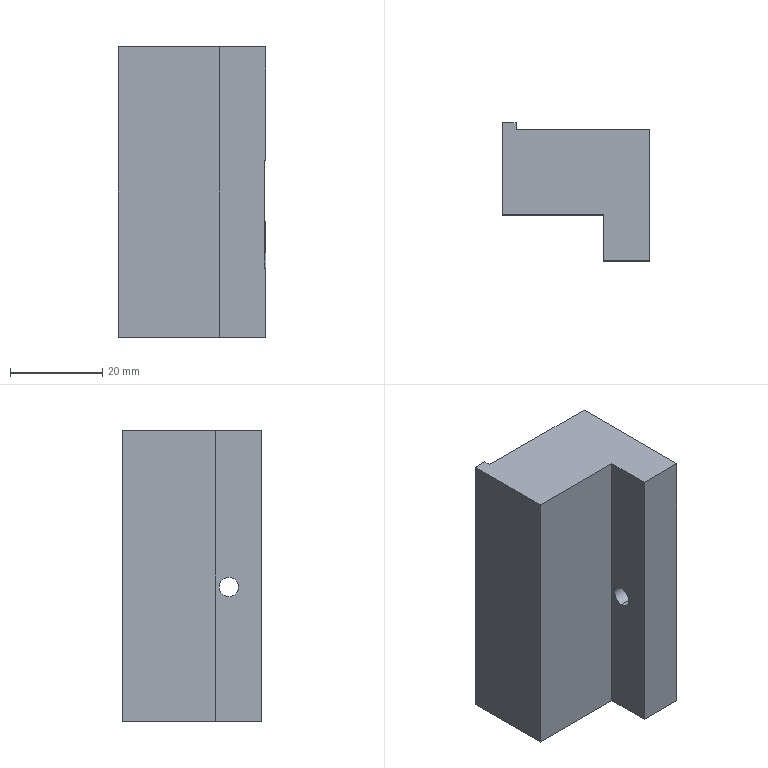Part | SolidWorks | features ICE 2, 3DProfileFeature 1, Extrusion 1, HoleWzd 1 | 1 solid | 16 faces | box 32 x 30 x 63 mm | volume 43546 mm3 | plane 14 | cylinder 2 | commonest cylinder face diameters 4.2 x2
STEP:
#1=CARTESIAN_POINT('',(22.,-23.,-0.2864));
#2=VERTEX_POINT('',#1);
#3=CARTESIAN_POINT('',(22.,-23.,-4.486));
#4=VERTEX_POINT('',#3);
#5=CARTESIAN_POINT('',(22.,-23.,-2.386));
#6=DIRECTION('',(1.,0.,0.));
#7=DIRECTION('',(0.,0.,-1.));
#8=AXIS2_PLACEMENT_3D('',#5,#6,#7);
#9=CIRCLE('',#8,2.1);
#10=EDGE_CURVE('',#2,#4,#9,.T.);
#11=ORIENTED_EDGE('',*,*,#10,.F.);
#12=CARTESIAN_POINT('',(31.7,-23.,-0.2864));
#13=VERTEX_POINT('',#12);
#14=CARTESIAN_POINT('',(31.7,-23.,-0.2864));
#15=DIRECTION('',(1.,0.,0.));
#16=VECTOR('',#15,1000.);
#17=LINE('',#14,#16);
#18=EDGE_CURVE('',#2,#13,#17,.T.);
#19=ORIENTED_EDGE('',*,*,#18,.T.);
#20=CARTESIAN_POINT('',(31.7,-23.,-4.486));
#21=VERTEX_POINT('',#20);
#22=CARTESIAN_POINT('',(31.7,-23.,-2.386));
#23=DIRECTION('',(1.,0.,0.));
#24=DIRECTION('',(0.,0.,-1.));
#25=AXIS2_PLACEMENT_3D('',#22,#23,#24);
#26=CIRCLE('',#25,2.1);
#27=EDGE_CURVE('',#13,#21,#26,.T.);
#28=ORIENTED_EDGE('',*,*,#27,.T.);
#29=CARTESIAN_POINT('',(31.7,-23.,-4.486));
#30=DIRECTION('',(1.,0.,0.));
#31=VECTOR('',#30,1000.);
#32=LINE('',#29,#31);
#33=EDGE_CURVE('',#4,#21,#32,.T.);
#34=ORIENTED_EDGE('',*,*,#33,.F.);
#35=EDGE_LOOP('',(#11,#19,#28,#34));
#36=FACE_OUTER_BOUND('',#35,.T.);
#37=CARTESIAN_POINT('',(31.7,-23.,-2.386));
#38=DIRECTION('',(1.,0.,0.));
#39=DIRECTION('',(0.,0.,-1.));
#40=AXIS2_PLACEMENT_3D('',#37,#38,#39);
#41=CYLINDRICAL_SURFACE('',#40,2.1);
#42=ADVANCED_FACE('',(#36),#41,.F.);
#43=CARTESIAN_POINT('',(32.,-1.5,-6.5));
#44=VERTEX_POINT('',#43);
#45=CARTESIAN_POINT('',(32.,-1.5,-31.5));
#46=VERTEX_POINT('',#45);
#47=CARTESIAN_POINT('',(32.,-1.5,-31.5));
#48=DIRECTION('',(0.,0.,-1.));
#49=VECTOR('',#48,1000.);
#50=LINE('',#47,#49);
#51=EDGE_CURVE('',#44,#46,#50,.T.);
#52=ORIENTED_EDGE('',*,*,#51,.F.);
#53=CARTESIAN_POINT('',(32.,-30.,-16.5));
#54=VERTEX_POINT('',#53);
#55=CARTESIAN_POINT('',(32.,-1.5,-6.5));
#56=DIRECTION('',(0.,0.9436,0.3311));
#57=VECTOR('',#56,1000.);
#58=LINE('',#55,#57);
#59=EDGE_CURVE('',#54,#44,#58,.T.);
#60=ORIENTED_EDGE('',*,*,#59,.F.);
#61=CARTESIAN_POINT('',(32.,-30.,-31.5));
#62=VERTEX_POINT('',#61);
#63=CARTESIAN_POINT('',(32.,-30.,31.5));
#64=DIRECTION('',(0.,0.,-1.));
#65=VECTOR('',#64,1000.);
#66=LINE('',#63,#65);
#67=EDGE_CURVE('',#54,#62,#66,.T.);
#68=ORIENTED_EDGE('',*,*,#67,.T.);
#69=CARTESIAN_POINT('',(32.,0.,-31.5));
#70=DIRECTION('',(0.,1.,0.));
#71=VECTOR('',#70,1000.);
#72=LINE('',#69,#71);
#73=EDGE_CURVE('',#62,#46,#72,.T.);
#74=ORIENTED_EDGE('',*,*,#73,.T.);
#75=EDGE_LOOP('',(#52,#60,#68,#74));
#76=FACE_OUTER_BOUND('',#75,.T.);
#77=CARTESIAN_POINT('',(32.,0.,31.5));
#78=DIRECTION('',(-1.,0.,0.));
#79=DIRECTION('',(0.,0.,1.));
#80=AXIS2_PLACEMENT_3D('',#77,#78,#79);
#81=PLANE('',#80);
#82=ADVANCED_FACE('',(#76),#81,.F.);
#83=CARTESIAN_POINT('',(0.,0.,-31.5));
#84=VERTEX_POINT('',#83);
#85=CARTESIAN_POINT('',(0.,-20.,-31.5));
#86=VERTEX_POINT('',#85);
#87=CARTESIAN_POINT('',(0.,-20.,-31.5));
#88=DIRECTION('',(0.,-1.,0.));
#89=VECTOR('',#88,1000.);
#90=LINE('',#87,#89);
#91=EDGE_CURVE('',#84,#86,#90,.T.);
#92=ORIENTED_EDGE('',*,*,#91,.T.);
#93=CARTESIAN_POINT('',(0.,-20.,31.5));
#94=VERTEX_POINT('',#93);
#95=CARTESIAN_POINT('',(0.,-20.,31.5));
#96=DIRECTION('',(0.,0.,-1.));
#97=VECTOR('',#96,1000.);
#98=LINE('',#95,#97);
#99=EDGE_CURVE('',#94,#86,#98,.T.);
#100=ORIENTED_EDGE('',*,*,#99,.F.);
#101=CARTESIAN_POINT('',(0.,0.,31.5));
#102=VERTEX_POINT('',#101);
#103=CARTESIAN_POINT('',(0.,-20.,31.5));
#104=DIRECTION('',(0.,-1.,0.));
#105=VECTOR('',#104,1000.);
#106=LINE('',#103,#105);
#107=EDGE_CURVE('',#102,#94,#106,.T.);
#108=ORIENTED_EDGE('',*,*,#107,.F.);
#109=CARTESIAN_POINT('',(0.,0.,31.5));
#110=DIRECTION('',(0.,0.,-1.));
#111=VECTOR('',#110,1000.);
#112=LINE('',#109,#111);
#113=EDGE_CURVE('',#102,#84,#112,.T.);
#114=ORIENTED_EDGE('',*,*,#113,.T.);
#115=EDGE_LOOP('',(#92,#100,#108,#114));
#116=FACE_OUTER_BOUND('',#115,.T.);
#117=CARTESIAN_POINT('',(0.,-20.,31.5));
#118=DIRECTION('',(1.,0.,0.));
#119=DIRECTION('',(0.,0.,-1.));
#120=AXIS2_PLACEMENT_3D('',#117,#118,#119);
#121=PLANE('',#120);
#122=ADVANCED_FACE('',(#116),#121,.F.);
#123=CARTESIAN_POINT('',(22.,-20.,-31.5));
#124=VERTEX_POINT('',#123);
#125=CARTESIAN_POINT('',(22.,-20.,-31.5));
#126=DIRECTION('',(1.,0.,0.));
#127=VECTOR('',#126,1000.);
#128=LINE('',#125,#127);
#129=EDGE_CURVE('',#86,#124,#128,.T.);
#130=ORIENTED_EDGE('',*,*,#129,.T.);
#131=CARTESIAN_POINT('',(22.,-20.,31.5));
#132=VERTEX_POINT('',#131);
#133=CARTESIAN_POINT('',(22.,-20.,31.5));
#134=DIRECTION('',(0.,0.,-1.));
#135=VECTOR('',#134,1000.);
#136=LINE('',#133,#135);
#137=EDGE_CURVE('',#132,#124,#136,.T.);
#138=ORIENTED_EDGE('',*,*,#137,.F.);
#139=CARTESIAN_POINT('',(22.,-20.,31.5));
#140=DIRECTION('',(1.,0.,0.));
#141=VECTOR('',#140,1000.);
#142=LINE('',#139,#141);
#143=EDGE_CURVE('',#94,#132,#142,.T.);
#144=ORIENTED_EDGE('',*,*,#143,.F.);
#145=ORIENTED_EDGE('',*,*,#99,.T.);
#146=EDGE_LOOP('',(#130,#138,#144,#145));
#147=FACE_OUTER_BOUND('',#146,.T.);
#148=CARTESIAN_POINT('',(22.,-20.,31.5));
#149=DIRECTION('',(0.,1.,0.));
#150=DIRECTION('',(-1.,0.,0.));
#151=AXIS2_PLACEMENT_3D('',#148,#149,#150);
#152=PLANE('',#151);
#153=ADVANCED_FACE('',(#147),#152,.F.);
#154=CARTESIAN_POINT('',(22.,-23.,-2.386));
#155=DIRECTION('',(1.,0.,0.));
#156=DIRECTION('',(0.,0.,-1.));
#157=AXIS2_PLACEMENT_3D('',#154,#155,#156);
#158=CIRCLE('',#157,2.1);
#159=EDGE_CURVE('',#4,#2,#158,.T.);
#160=ORIENTED_EDGE('',*,*,#159,.T.);
#161=ORIENTED_EDGE('',*,*,#10,.T.);
#162=EDGE_LOOP('',(#160,#161));
#163=FACE_BOUND('',#162,.T.);
#164=CARTESIAN_POINT('',(22.,-30.,-31.5));
#165=VERTEX_POINT('',#164);
#166=CARTESIAN_POINT('',(22.,-30.,-31.5));
#167=DIRECTION('',(0.,-1.,0.));
#168=VECTOR('',#167,1000.);
#169=LINE('',#166,#168);
#170=EDGE_CURVE('',#124,#165,#169,.T.);
#171=ORIENTED_EDGE('',*,*,#170,.T.);
#172=CARTESIAN_POINT('',(22.,-30.,31.5));
#173=VERTEX_POINT('',#172);
#174=CARTESIAN_POINT('',(22.,-30.,31.5));
#175=DIRECTION('',(0.,0.,-1.));
#176=VECTOR('',#175,1000.);
#177=LINE('',#174,#176);
#178=EDGE_CURVE('',#173,#165,#177,.T.);
#179=ORIENTED_EDGE('',*,*,#178,.F.);
#180=CARTESIAN_POINT('',(22.,-30.,31.5));
#181=DIRECTION('',(0.,-1.,0.));
#182=VECTOR('',#181,1000.);
#183=LINE('',#180,#182);
#184=EDGE_CURVE('',#132,#173,#183,.T.);
#185=ORIENTED_EDGE('',*,*,#184,.F.);
#186=ORIENTED_EDGE('',*,*,#137,.T.);
#187=EDGE_LOOP('',(#171,#179,#185,#186));
#188=FACE_OUTER_BOUND('',#187,.T.);
#189=CARTESIAN_POINT('',(22.,-30.,31.5));
#190=DIRECTION('',(1.,0.,0.));
#191=DIRECTION('',(0.,0.,-1.));
#192=AXIS2_PLACEMENT_3D('',#189,#190,#191);
#193=PLANE('',#192);
#194=ADVANCED_FACE('',(#163,#188),#193,.F.);
#195=ORIENTED_EDGE('',*,*,#67,.F.);
#196=CARTESIAN_POINT('',(31.7,-30.,-16.5));
#197=VERTEX_POINT('',#196);
#198=CARTESIAN_POINT('',(31.7,-30.,-16.5));
#199=DIRECTION('',(1.,0.,0.));
#200=VECTOR('',#199,1000.);
#201=LINE('',#198,#200);
#202=EDGE_CURVE('',#197,#54,#201,.T.);
#203=ORIENTED_EDGE('',*,*,#202,.F.);
#204=CARTESIAN_POINT('',(31.7,-30.,6.815));
#205=VERTEX_POINT('',#204);
#206=CARTESIAN_POINT('',(31.7,-30.,-16.5));
#207=DIRECTION('',(0.,0.,-1.));
#208=VECTOR('',#207,1000.);
#209=LINE('',#206,#208);
#210=EDGE_CURVE('',#205,#197,#209,.T.);
#211=ORIENTED_EDGE('',*,*,#210,.F.);
#212=CARTESIAN_POINT('',(32.,-30.,6.815));
#213=VERTEX_POINT('',#212);
#214=CARTESIAN_POINT('',(31.7,-30.,6.815));
#215=DIRECTION('',(1.,0.,0.));
#216=VECTOR('',#215,1000.);
#217=LINE('',#214,#216);
#218=EDGE_CURVE('',#205,#213,#217,.T.);
#219=ORIENTED_EDGE('',*,*,#218,.T.);
#220=CARTESIAN_POINT('',(32.,-30.,31.5));
#221=VERTEX_POINT('',#220);
#222=CARTESIAN_POINT('',(32.,-30.,31.5));
#223=DIRECTION('',(0.,0.,-1.));
#224=VECTOR('',#223,1000.);
#225=LINE('',#222,#224);
#226=EDGE_CURVE('',#221,#213,#225,.T.);
#227=ORIENTED_EDGE('',*,*,#226,.F.);
#228=CARTESIAN_POINT('',(32.,-30.,31.5));
#229=DIRECTION('',(1.,0.,0.));
#230=VECTOR('',#229,1000.);
#231=LINE('',#228,#230);
#232=EDGE_CURVE('',#173,#221,#231,.T.);
#233=ORIENTED_EDGE('',*,*,#232,.F.);
#234=ORIENTED_EDGE('',*,*,#178,.T.);
#235=CARTESIAN_POINT('',(32.,-30.,-31.5));
#236=DIRECTION('',(1.,0.,0.));
#237=VECTOR('',#236,1000.);
#238=LINE('',#235,#237);
#239=EDGE_CURVE('',#165,#62,#238,.T.);
#240=ORIENTED_EDGE('',*,*,#239,.T.);
#241=EDGE_LOOP('',(#195,#203,#211,#219,#227,#233,#234,#240));
#242=FACE_OUTER_BOUND('',#241,.T.);
#243=CARTESIAN_POINT('',(32.,-30.,31.5));
#244=DIRECTION('',(0.,1.,0.));
#245=DIRECTION('',(0.,0.,1.));
#246=AXIS2_PLACEMENT_3D('',#243,#244,#245);
#247=PLANE('',#246);
#248=ADVANCED_FACE('',(#242),#247,.F.);
#249=ORIENTED_EDGE('',*,*,#226,.T.);
#250=CARTESIAN_POINT('',(32.,-1.5,16.815));
#251=VERTEX_POINT('',#250);
#252=CARTESIAN_POINT('',(32.,-1.5,16.815));
#253=DIRECTION('',(0.,-0.9436,-0.3311));
#254=VECTOR('',#253,1000.);
#255=LINE('',#252,#254);
#256=EDGE_CURVE('',#251,#213,#255,.T.);
#257=ORIENTED_EDGE('',*,*,#256,.F.);
#258=CARTESIAN_POINT('',(32.,-1.5,31.5));
#259=VERTEX_POINT('',#258);
#260=CARTESIAN_POINT('',(32.,-1.5,-31.5));
#261=DIRECTION('',(0.,0.,-1.));
#262=VECTOR('',#261,1000.);
#263=LINE('',#260,#262);
#264=EDGE_CURVE('',#259,#251,#263,.T.);
#265=ORIENTED_EDGE('',*,*,#264,.F.);
#266=CARTESIAN_POINT('',(32.,0.,31.5));
#267=DIRECTION('',(0.,1.,0.));
#268=VECTOR('',#267,1000.);
#269=LINE('',#266,#268);
#270=EDGE_CURVE('',#221,#259,#269,.T.);
#271=ORIENTED_EDGE('',*,*,#270,.F.);
#272=EDGE_LOOP('',(#249,#257,#265,#271));
#273=FACE_OUTER_BOUND('',#272,.T.);
#274=CARTESIAN_POINT('',(32.,0.,31.5));
#275=DIRECTION('',(-1.,0.,0.));
#276=DIRECTION('',(0.,0.,1.));
#277=AXIS2_PLACEMENT_3D('',#274,#275,#276);
#278=PLANE('',#277);
#279=ADVANCED_FACE('',(#273),#278,.F.);
#280=CARTESIAN_POINT('',(3.,0.,31.5));
#281=VERTEX_POINT('',#280);
#282=CARTESIAN_POINT('',(0.,0.,31.5));
#283=DIRECTION('',(-1.,0.,0.));
#284=VECTOR('',#283,1000.);
#285=LINE('',#282,#284);
#286=EDGE_CURVE('',#281,#102,#285,.T.);
#287=ORIENTED_EDGE('',*,*,#286,.F.);
#288=CARTESIAN_POINT('',(3.,0.,-31.5));
#289=VERTEX_POINT('',#288);
#290=CARTESIAN_POINT('',(3.,0.,-31.5));
#291=DIRECTION('',(0.,0.,1.));
#292=VECTOR('',#291,1000.);
#293=LINE('',#290,#292);
#294=EDGE_CURVE('',#289,#281,#293,.T.);
#295=ORIENTED_EDGE('',*,*,#294,.F.);
#296=CARTESIAN_POINT('',(0.,0.,-31.5));
#297=DIRECTION('',(-1.,0.,0.));
#298=VECTOR('',#297,1000.);
#299=LINE('',#296,#298);
#300=EDGE_CURVE('',#289,#84,#299,.T.);
#301=ORIENTED_EDGE('',*,*,#300,.T.);
#302=ORIENTED_EDGE('',*,*,#113,.F.);
#303=EDGE_LOOP('',(#287,#295,#301,#302));
#304=FACE_OUTER_BOUND('',#303,.T.);
#305=CARTESIAN_POINT('',(0.,0.,31.5));
#306=DIRECTION('',(0.,-1.,0.));
#307=DIRECTION('',(0.,0.,-1.));
#308=AXIS2_PLACEMENT_3D('',#305,#306,#307);
#309=PLANE('',#308);
#310=ADVANCED_FACE('',(#304),#309,.F.);
#311=CARTESIAN_POINT('',(3.,-1.5,31.5));
#312=VERTEX_POINT('',#311);
#313=CARTESIAN_POINT('',(32.,-1.5,31.5));
#314=DIRECTION('',(1.,0.,0.));
#315=VECTOR('',#314,1000.);
#316=LINE('',#313,#315);
#317=EDGE_CURVE('',#312,#259,#316,.T.);
#318=ORIENTED_EDGE('',*,*,#317,.F.);
#319=CARTESIAN_POINT('',(3.,-1.5,31.5));
#320=DIRECTION('',(0.,1.,0.));
#321=VECTOR('',#320,1000.);
#322=LINE('',#319,#321);
#323=EDGE_CURVE('',#312,#281,#322,.T.);
#324=ORIENTED_EDGE('',*,*,#323,.T.);
#325=ORIENTED_EDGE('',*,*,#286,.T.);
#326=ORIENTED_EDGE('',*,*,#107,.T.);
#327=ORIENTED_EDGE('',*,*,#143,.T.);
#328=ORIENTED_EDGE('',*,*,#184,.T.);
#329=ORIENTED_EDGE('',*,*,#232,.T.);
#330=ORIENTED_EDGE('',*,*,#270,.T.);
#331=EDGE_LOOP('',(#318,#324,#325,#326,#327,#328,#329,#330));
#332=FACE_OUTER_BOUND('',#331,.T.);
#333=CARTESIAN_POINT('',(0.,0.,31.5));
#334=DIRECTION('',(0.,0.,-1.));
#335=DIRECTION('',(-1.,0.,0.));
#336=AXIS2_PLACEMENT_3D('',#333,#334,#335);
#337=PLANE('',#336);
#338=ADVANCED_FACE('',(#332),#337,.F.);
#339=CARTESIAN_POINT('',(3.,-1.5,-31.5));
#340=VERTEX_POINT('',#339);
#341=CARTESIAN_POINT('',(3.,-1.5,-31.5));
#342=DIRECTION('',(0.,1.,0.));
#343=VECTOR('',#342,1000.);
#344=LINE('',#341,#343);
#345=EDGE_CURVE('',#340,#289,#344,.T.);
#346=ORIENTED_EDGE('',*,*,#345,.F.);
#347=CARTESIAN_POINT('',(32.,-1.5,-31.5));
#348=DIRECTION('',(-1.,0.,0.));
#349=VECTOR('',#348,1000.);
#350=LINE('',#347,#349);
#351=EDGE_CURVE('',#46,#340,#350,.T.);
#352=ORIENTED_EDGE('',*,*,#351,.F.);
#353=ORIENTED_EDGE('',*,*,#73,.F.);
#354=ORIENTED_EDGE('',*,*,#239,.F.);
#355=ORIENTED_EDGE('',*,*,#170,.F.);
#356=ORIENTED_EDGE('',*,*,#129,.F.);
#357=ORIENTED_EDGE('',*,*,#91,.F.);
#358=ORIENTED_EDGE('',*,*,#300,.F.);
#359=EDGE_LOOP('',(#346,#352,#353,#354,#355,#356,#357,#358));
#360=FACE_OUTER_BOUND('',#359,.T.);
#361=CARTESIAN_POINT('',(0.,0.,-31.5));
#362=DIRECTION('',(0.,0.,-1.));
#363=DIRECTION('',(-1.,0.,0.));
#364=AXIS2_PLACEMENT_3D('',#361,#362,#363);
#365=PLANE('',#364);
#366=ADVANCED_FACE('',(#360),#365,.T.);
#367=ORIENTED_EDGE('',*,*,#294,.T.);
#368=ORIENTED_EDGE('',*,*,#323,.F.);
#369=CARTESIAN_POINT('',(3.,-1.5,-31.5));
#370=DIRECTION('',(0.,0.,1.));
#371=VECTOR('',#370,1000.);
#372=LINE('',#369,#371);
#373=EDGE_CURVE('',#340,#312,#372,.T.);
#374=ORIENTED_EDGE('',*,*,#373,.F.);
#375=ORIENTED_EDGE('',*,*,#345,.T.);
#376=EDGE_LOOP('',(#367,#368,#374,#375));
#377=FACE_OUTER_BOUND('',#376,.T.);
#378=CARTESIAN_POINT('',(3.,-1.5,-31.5));
#379=DIRECTION('',(-1.,0.,0.));
#380=DIRECTION('',(0.,0.,1.));
#381=AXIS2_PLACEMENT_3D('',#378,#379,#380);
#382=PLANE('',#381);
#383=ADVANCED_FACE('',(#377),#382,.F.);
#384=CARTESIAN_POINT('',(31.7,-1.5,-6.5));
#385=VERTEX_POINT('',#384);
#386=CARTESIAN_POINT('',(31.7,-1.5,16.815));
#387=VERTEX_POINT('',#386);
#388=CARTESIAN_POINT('',(31.7,-1.5,16.815));
#389=DIRECTION('',(0.,0.,1.));
#390=VECTOR('',#389,1000.);
#391=LINE('',#388,#390);
#392=EDGE_CURVE('',#385,#387,#391,.T.);
#393=ORIENTED_EDGE('',*,*,#392,.F.);
#394=CARTESIAN_POINT('',(31.7,-1.5,-6.5));
#395=DIRECTION('',(1.,0.,0.));
#396=VECTOR('',#395,1000.);
#397=LINE('',#394,#396);
#398=EDGE_CURVE('',#385,#44,#397,.T.);
#399=ORIENTED_EDGE('',*,*,#398,.T.);
#400=ORIENTED_EDGE('',*,*,#51,.T.);
#401=ORIENTED_EDGE('',*,*,#351,.T.);
#402=ORIENTED_EDGE('',*,*,#373,.T.);
#403=ORIENTED_EDGE('',*,*,#317,.T.);
#404=ORIENTED_EDGE('',*,*,#264,.T.);
#405=CARTESIAN_POINT('',(31.7,-1.5,16.815));
#406=DIRECTION('',(1.,0.,0.));
#407=VECTOR('',#406,1000.);
#408=LINE('',#405,#407);
#409=EDGE_CURVE('',#387,#251,#408,.T.);
#410=ORIENTED_EDGE('',*,*,#409,.F.);
#411=EDGE_LOOP('',(#393,#399,#400,#401,#402,#403,#404,#410));
#412=FACE_OUTER_BOUND('',#411,.T.);
#413=CARTESIAN_POINT('',(0.,-1.5,0.));
#414=DIRECTION('',(0.,-1.,0.));
#415=DIRECTION('',(0.,0.,-1.));
#416=AXIS2_PLACEMENT_3D('',#413,#414,#415);
#417=PLANE('',#416);
#418=ADVANCED_FACE('',(#412),#417,.F.);
#419=ORIENTED_EDGE('',*,*,#59,.T.);
#420=ORIENTED_EDGE('',*,*,#398,.F.);
#421=CARTESIAN_POINT('',(31.7,-1.5,-6.5));
#422=DIRECTION('',(0.,0.9436,0.3311));
#423=VECTOR('',#422,1000.);
#424=LINE('',#421,#423);
#425=EDGE_CURVE('',#197,#385,#424,.T.);
#426=ORIENTED_EDGE('',*,*,#425,.F.);
#427=ORIENTED_EDGE('',*,*,#202,.T.);
#428=EDGE_LOOP('',(#419,#420,#426,#427));
#429=FACE_OUTER_BOUND('',#428,.T.);
#430=CARTESIAN_POINT('',(31.7,-1.5,-6.5));
#431=DIRECTION('',(0.,0.3311,-0.9436));
#432=DIRECTION('',(0.,0.9436,0.3311));
#433=AXIS2_PLACEMENT_3D('',#430,#431,#432);
#434=PLANE('',#433);
#435=ADVANCED_FACE('',(#429),#434,.F.);
#436=ORIENTED_EDGE('',*,*,#256,.T.);
#437=ORIENTED_EDGE('',*,*,#218,.F.);
#438=CARTESIAN_POINT('',(31.7,-1.5,16.815));
#439=DIRECTION('',(0.,-0.9436,-0.3311));
#440=VECTOR('',#439,1000.);
#441=LINE('',#438,#440);
#442=EDGE_CURVE('',#387,#205,#441,.T.);
#443=ORIENTED_EDGE('',*,*,#442,.F.);
#444=ORIENTED_EDGE('',*,*,#409,.T.);
#445=EDGE_LOOP('',(#436,#437,#443,#444));
#446=FACE_OUTER_BOUND('',#445,.T.);
#447=CARTESIAN_POINT('',(31.7,-1.5,16.815));
#448=DIRECTION('',(0.,-0.3311,0.9436));
#449=DIRECTION('',(0.,-0.9436,-0.3311));
#450=AXIS2_PLACEMENT_3D('',#447,#448,#449);
#451=PLANE('',#450);
#452=ADVANCED_FACE('',(#446),#451,.F.);
#453=CARTESIAN_POINT('',(31.7,-23.,-2.386));
#454=DIRECTION('',(1.,0.,0.));
#455=DIRECTION('',(0.,0.,-1.));
#456=AXIS2_PLACEMENT_3D('',#453,#454,#455);
#457=CIRCLE('',#456,2.1);
#458=EDGE_CURVE('',#21,#13,#457,.T.);
#459=ORIENTED_EDGE('',*,*,#458,.F.);
#460=ORIENTED_EDGE('',*,*,#27,.F.);
#461=EDGE_LOOP('',(#459,#460));
#462=FACE_BOUND('',#461,.T.);
#463=ORIENTED_EDGE('',*,*,#392,.T.);
#464=ORIENTED_EDGE('',*,*,#442,.T.);
#465=ORIENTED_EDGE('',*,*,#210,.T.);
#466=ORIENTED_EDGE('',*,*,#425,.T.);
#467=EDGE_LOOP('',(#463,#464,#465,#466));
#468=FACE_OUTER_BOUND('',#467,.T.);
#469=CARTESIAN_POINT('',(31.7,0.,0.));
#470=DIRECTION('',(-1.,0.,0.));
#471=DIRECTION('',(0.,0.,1.));
#472=AXIS2_PLACEMENT_3D('',#469,#470,#471);
#473=PLANE('',#472);
#474=ADVANCED_FACE('',(#462,#468),#473,.F.);
#475=ORIENTED_EDGE('',*,*,#18,.F.);
#476=ORIENTED_EDGE('',*,*,#159,.F.);
#477=ORIENTED_EDGE('',*,*,#33,.T.);
#478=ORIENTED_EDGE('',*,*,#458,.T.);
#479=EDGE_LOOP('',(#475,#476,#477,#478));
#480=FACE_OUTER_BOUND('',#479,.T.);
#481=CARTESIAN_POINT('',(31.7,-23.,-2.386));
#482=DIRECTION('',(1.,0.,0.));
#483=DIRECTION('',(0.,0.,-1.));
#484=AXIS2_PLACEMENT_3D('',#481,#482,#483);
#485=CYLINDRICAL_SURFACE('',#484,2.1);
#486=ADVANCED_FACE('',(#480),#485,.F.);
#487=CLOSED_SHELL('',(#42,#82,#122,#153,#194,#248,#279,#310,#338,#366,#383,#418,#435,#452,#474,#486));
#488=MANIFOLD_SOLID_BREP('',#487);
#489=CARTESIAN_POINT('',(0.,0.,0.));
#490=DIRECTION('',(0.,0.,1.));
#491=DIRECTION('',(1.,0.,0.));
#492=AXIS2_PLACEMENT_3D('',#489,#490,#491);
#493=(LENGTH_UNIT()NAMED_UNIT(*)SI_UNIT(.MILLI.,.METRE.));
#494=UNCERTAINTY_MEASURE_WITH_UNIT(LENGTH_MEASURE(0.00001),#493,'','');
#495=(NAMED_UNIT(*)PLANE_ANGLE_UNIT()SI_UNIT($,.RADIAN.));
#496=(NAMED_UNIT(*)SI_UNIT($,.STERADIAN.)SOLID_ANGLE_UNIT());
#497=(GEOMETRIC_REPRESENTATION_CONTEXT(3)GLOBAL_UNCERTAINTY_ASSIGNED_CONTEXT((#494))GLOBAL_UNIT_ASSIGNED_CONTEXT((#493,#495,#496))REPRESENTATION_CONTEXT('',''));
#498=ADVANCED_BREP_SHAPE_REPRESENTATION('',(#488,#492),#497);